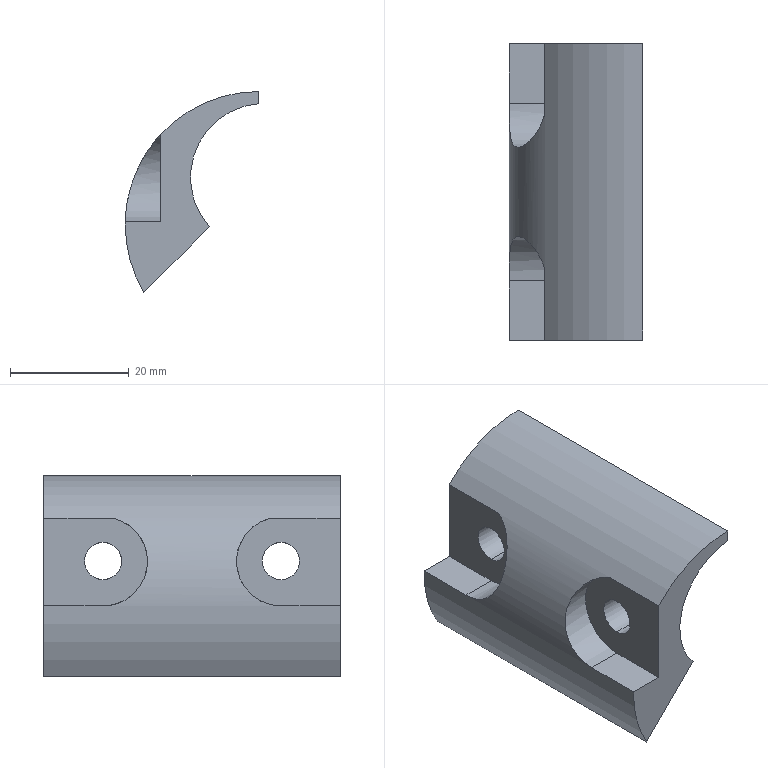Part | SolidWorks | features BaseBody 1 | 1 solid | 16 faces | box 22.5 x 50 x 33.899 mm | volume 12325 mm3 | cylinder 8 | plane 8 | commonest cylinder face diameters 6.3 x4 15 x2 25 x1 45 x1
STEP:
#1=CARTESIAN_POINT('',(909.83,-3885.973,891.894));
#2=VERTEX_POINT('',#1);
#3=CARTESIAN_POINT('',(909.868,-3885.973,898.194));
#4=VERTEX_POINT('',#3);
#5=CARTESIAN_POINT('',(909.83,-3885.973,891.894));
#6=CARTESIAN_POINT('',(909.83,-3886.182,891.894));
#7=CARTESIAN_POINT('',(909.825,-3886.387,891.915));
#8=CARTESIAN_POINT('',(909.805,-3886.791,891.995));
#9=CARTESIAN_POINT('',(909.79,-3886.992,892.056));
#10=CARTESIAN_POINT('',(909.753,-3887.373,892.214));
#11=CARTESIAN_POINT('',(909.731,-3887.553,892.311));
#12=CARTESIAN_POINT('',(909.684,-3887.895,892.54));
#13=CARTESIAN_POINT('',(909.658,-3888.056,892.672));
#14=CARTESIAN_POINT('',(909.607,-3888.346,892.962));
#15=CARTESIAN_POINT('',(909.582,-3888.476,893.12));
#16=CARTESIAN_POINT('',(909.536,-3888.706,893.464));
#17=CARTESIAN_POINT('',(909.515,-3888.804,893.646));
#18=CARTESIAN_POINT('',(909.48,-3888.961,894.025));
#19=CARTESIAN_POINT('',(909.466,-3889.022,894.225));
#20=CARTESIAN_POINT('',(909.448,-3889.103,894.632));
#21=CARTESIAN_POINT('',(909.444,-3889.123,894.839));
#22=CARTESIAN_POINT('',(909.447,-3889.123,895.257));
#23=CARTESIAN_POINT('',(909.454,-3889.102,895.462));
#24=CARTESIAN_POINT('',(909.476,-3889.021,895.866));
#25=CARTESIAN_POINT('',(909.492,-3888.96,896.066));
#26=CARTESIAN_POINT('',(909.531,-3888.801,896.447));
#27=CARTESIAN_POINT('',(909.554,-3888.704,896.627));
#28=CARTESIAN_POINT('',(909.605,-3888.475,896.968));
#29=CARTESIAN_POINT('',(909.632,-3888.343,897.129));
#30=CARTESIAN_POINT('',(909.686,-3888.053,897.418));
#31=CARTESIAN_POINT('',(909.713,-3887.895,897.548));
#32=CARTESIAN_POINT('',(909.764,-3887.551,897.778));
#33=CARTESIAN_POINT('',(909.787,-3887.369,897.875));
#34=CARTESIAN_POINT('',(909.826,-3886.991,898.032));
#35=CARTESIAN_POINT('',(909.841,-3886.791,898.093));
#36=CARTESIAN_POINT('',(909.863,-3886.384,898.174));
#37=CARTESIAN_POINT('',(909.868,-3886.179,898.194));
#38=CARTESIAN_POINT('',(909.868,-3885.973,898.194));
#39=B_SPLINE_CURVE_WITH_KNOTS('',3,(#5,#6,#7,#8,#9,#10,#11,#12,#13,#14,#15,#16,#17,#18,#19,#20,#21,#22,#23,#24,#25,#26,#27,#28,#29,#30,#31,#32,#33,#34,#35,#36,#37,#38),.UNSPECIFIED.,.F.,.F.,(4,2,2,2,2,2,2,2,2,2,2,2,2,2,2,2,4),(0.,0.0006179,0.001236,0.001854,0.002472,0.00309,0.003707,0.004325,0.004943,0.005561,0.006179,0.006797,0.007415,0.008033,0.008651,0.009269,0.009886),.UNSPECIFIED.);
#40=EDGE_CURVE('',#2,#4,#39,.T.);
#41=ORIENTED_EDGE('',*,*,#40,.F.);
#42=CARTESIAN_POINT('',(904.446,-3885.973,891.894));
#43=VERTEX_POINT('',#42);
#44=CARTESIAN_POINT('',(894.755,-3885.973,891.894));
#45=DIRECTION('',(-1.,0.,0.));
#46=VECTOR('',#45,1000.);
#47=LINE('',#44,#46);
#48=EDGE_CURVE('',#2,#43,#47,.T.);
#49=ORIENTED_EDGE('',*,*,#48,.T.);
#50=CARTESIAN_POINT('',(904.446,-3885.973,898.194));
#51=VERTEX_POINT('',#50);
#52=CARTESIAN_POINT('',(904.446,-3885.973,895.044));
#53=DIRECTION('',(-1.,0.,0.));
#54=DIRECTION('',(0.,0.,1.));
#55=AXIS2_PLACEMENT_3D('',#52,#53,#54);
#56=CIRCLE('',#55,3.15);
#57=EDGE_CURVE('',#43,#51,#56,.T.);
#58=ORIENTED_EDGE('',*,*,#57,.T.);
#59=CARTESIAN_POINT('',(894.755,-3885.973,898.194));
#60=DIRECTION('',(-1.,0.,0.));
#61=VECTOR('',#60,1000.);
#62=LINE('',#59,#61);
#63=EDGE_CURVE('',#4,#51,#62,.T.);
#64=ORIENTED_EDGE('',*,*,#63,.F.);
#65=EDGE_LOOP('',(#41,#49,#58,#64));
#66=FACE_OUTER_BOUND('',#65,.T.);
#67=CARTESIAN_POINT('',(894.755,-3885.973,895.044));
#68=DIRECTION('',(-1.,0.,0.));
#69=DIRECTION('',(0.,0.,1.));
#70=AXIS2_PLACEMENT_3D('',#67,#68,#69);
#71=CYLINDRICAL_SURFACE('',#70,3.15);
#72=ADVANCED_FACE('',(#66),#71,.F.);
#73=CARTESIAN_POINT('',(904.446,-3915.973,891.894));
#74=VERTEX_POINT('',#73);
#75=CARTESIAN_POINT('',(904.446,-3915.973,898.194));
#76=VERTEX_POINT('',#75);
#77=CARTESIAN_POINT('',(904.446,-3915.973,895.044));
#78=DIRECTION('',(-1.,0.,0.));
#79=DIRECTION('',(0.,0.,-1.));
#80=AXIS2_PLACEMENT_3D('',#77,#78,#79);
#81=CIRCLE('',#80,3.15);
#82=EDGE_CURVE('',#74,#76,#81,.T.);
#83=ORIENTED_EDGE('',*,*,#82,.T.);
#84=CARTESIAN_POINT('',(909.868,-3915.973,898.194));
#85=VERTEX_POINT('',#84);
#86=CARTESIAN_POINT('',(894.755,-3915.973,898.194));
#87=DIRECTION('',(1.,0.,0.));
#88=VECTOR('',#87,1000.);
#89=LINE('',#86,#88);
#90=EDGE_CURVE('',#76,#85,#89,.T.);
#91=ORIENTED_EDGE('',*,*,#90,.T.);
#92=CARTESIAN_POINT('',(909.83,-3915.973,891.894));
#93=VERTEX_POINT('',#92);
#94=CARTESIAN_POINT('',(909.83,-3915.973,891.894));
#95=CARTESIAN_POINT('',(909.83,-3916.179,891.894));
#96=CARTESIAN_POINT('',(909.825,-3916.389,891.915));
#97=CARTESIAN_POINT('',(909.805,-3916.793,891.996));
#98=CARTESIAN_POINT('',(909.79,-3916.99,892.055));
#99=CARTESIAN_POINT('',(909.735,-3917.563,892.293));
#100=CARTESIAN_POINT('',(909.684,-3917.909,892.525));
#101=CARTESIAN_POINT('',(909.607,-3918.347,892.963));
#102=CARTESIAN_POINT('',(909.582,-3918.476,893.121));
#103=CARTESIAN_POINT('',(909.536,-3918.704,893.461));
#104=CARTESIAN_POINT('',(909.515,-3918.803,893.646));
#105=CARTESIAN_POINT('',(909.48,-3918.961,894.026));
#106=CARTESIAN_POINT('',(909.466,-3919.021,894.222));
#107=CARTESIAN_POINT('',(909.449,-3919.102,894.628));
#108=CARTESIAN_POINT('',(909.445,-3919.123,894.837));
#109=CARTESIAN_POINT('',(909.447,-3919.123,895.255));
#110=CARTESIAN_POINT('',(909.453,-3919.102,895.46));
#111=CARTESIAN_POINT('',(909.476,-3919.022,895.863));
#112=CARTESIAN_POINT('',(909.492,-3918.961,896.064));
#113=CARTESIAN_POINT('',(909.531,-3918.802,896.444));
#114=CARTESIAN_POINT('',(909.554,-3918.706,896.625));
#115=CARTESIAN_POINT('',(909.604,-3918.477,896.966));
#116=CARTESIAN_POINT('',(909.632,-3918.345,897.127));
#117=CARTESIAN_POINT('',(909.686,-3918.056,897.416));
#118=CARTESIAN_POINT('',(909.713,-3917.898,897.546));
#119=CARTESIAN_POINT('',(909.764,-3917.555,897.776));
#120=CARTESIAN_POINT('',(909.787,-3917.373,897.873));
#121=CARTESIAN_POINT('',(909.825,-3916.995,898.031));
#122=CARTESIAN_POINT('',(909.841,-3916.796,898.092));
#123=CARTESIAN_POINT('',(909.863,-3916.388,898.173));
#124=CARTESIAN_POINT('',(909.868,-3916.182,898.194));
#125=CARTESIAN_POINT('',(909.868,-3915.973,898.194));
#126=B_SPLINE_CURVE_WITH_KNOTS('',3,(#94,#95,#96,#97,#98,#99,#100,#101,#102,#103,#104,#105,#106,#107,#108,#109,#110,#111,#112,#113,#114,#115,#116,#117,#118,#119,#120,#121,#122,#123,#124,#125),.UNSPECIFIED.,.F.,.F.,(4,2,2,2,2,2,2,2,2,2,2,2,2,2,2,4),(-0.004938,-0.004321,-0.003703,-0.002468,-0.001851,-0.001233,-0.0006155,0.000002039,0.0006196,0.001237,0.001855,0.002472,0.00309,0.003707,0.004325,0.004942),.UNSPECIFIED.);
#127=EDGE_CURVE('',#93,#85,#126,.T.);
#128=ORIENTED_EDGE('',*,*,#127,.F.);
#129=CARTESIAN_POINT('',(894.755,-3915.973,891.894));
#130=DIRECTION('',(1.,0.,0.));
#131=VECTOR('',#130,1000.);
#132=LINE('',#129,#131);
#133=EDGE_CURVE('',#74,#93,#132,.T.);
#134=ORIENTED_EDGE('',*,*,#133,.F.);
#135=EDGE_LOOP('',(#83,#91,#128,#134));
#136=FACE_OUTER_BOUND('',#135,.T.);
#137=CARTESIAN_POINT('',(894.755,-3915.973,895.044));
#138=DIRECTION('',(1.,0.,0.));
#139=DIRECTION('',(0.,0.,-1.));
#140=AXIS2_PLACEMENT_3D('',#137,#138,#139);
#141=CYLINDRICAL_SURFACE('',#140,3.15);
#142=ADVANCED_FACE('',(#136),#141,.F.);
#143=CARTESIAN_POINT('',(904.446,-3875.973,902.268));
#144=VERTEX_POINT('',#143);
#145=CARTESIAN_POINT('',(904.446,-3887.706,902.268));
#146=VERTEX_POINT('',#145);
#147=CARTESIAN_POINT('',(904.446,-3875.973,902.268));
#148=DIRECTION('',(0.,-1.,0.));
#149=VECTOR('',#148,1000.);
#150=LINE('',#147,#149);
#151=EDGE_CURVE('',#144,#146,#150,.T.);
#152=ORIENTED_EDGE('',*,*,#151,.T.);
#153=CARTESIAN_POINT('',(898.451,-3885.973,887.471));
#154=VERTEX_POINT('',#153);
#155=CARTESIAN_POINT('',(904.446,-3887.706,902.268));
#156=CARTESIAN_POINT('',(904.344,-3888.167,902.159));
#157=CARTESIAN_POINT('',(904.209,-3888.6,902.011));
#158=CARTESIAN_POINT('',(903.969,-3889.215,901.738));
#159=CARTESIAN_POINT('',(903.883,-3889.414,901.639));
#160=CARTESIAN_POINT('',(903.701,-3889.802,901.424));
#161=CARTESIAN_POINT('',(903.604,-3889.991,901.308));
#162=CARTESIAN_POINT('',(903.305,-3890.534,900.941));
#163=CARTESIAN_POINT('',(903.093,-3890.867,900.671));
#164=CARTESIAN_POINT('',(902.655,-3891.481,900.08));
#165=CARTESIAN_POINT('',(902.427,-3891.763,899.758));
#166=CARTESIAN_POINT('',(901.976,-3892.263,899.079));
#167=CARTESIAN_POINT('',(901.752,-3892.483,898.721));
#168=CARTESIAN_POINT('',(901.309,-3892.863,897.965));
#169=CARTESIAN_POINT('',(901.089,-3893.024,897.563));
#170=CARTESIAN_POINT('',(900.672,-3893.274,896.74));
#171=CARTESIAN_POINT('',(900.473,-3893.364,896.318));
#172=CARTESIAN_POINT('',(900.193,-3893.444,895.668));
#173=CARTESIAN_POINT('',(900.102,-3893.461,895.449));
#174=CARTESIAN_POINT('',(899.927,-3893.476,895.004));
#175=CARTESIAN_POINT('',(899.842,-3893.474,894.777));
#176=CARTESIAN_POINT('',(899.599,-3893.436,894.099));
#177=CARTESIAN_POINT('',(899.455,-3893.37,893.65));
#178=CARTESIAN_POINT('',(899.262,-3893.208,892.983));
#179=CARTESIAN_POINT('',(899.202,-3893.144,892.762));
#180=CARTESIAN_POINT('',(899.09,-3892.994,892.322));
#181=CARTESIAN_POINT('',(899.037,-3892.907,892.102));
#182=CARTESIAN_POINT('',(898.893,-3892.615,891.457));
#183=CARTESIAN_POINT('',(898.814,-3892.382,891.048));
#184=CARTESIAN_POINT('',(898.718,-3891.975,890.467));
#185=CARTESIAN_POINT('',(898.689,-3891.829,890.28));
#186=CARTESIAN_POINT('',(898.638,-3891.518,889.916));
#187=CARTESIAN_POINT('',(898.616,-3891.352,889.74));
#188=CARTESIAN_POINT('',(898.558,-3890.836,889.242));
#189=CARTESIAN_POINT('',(898.531,-3890.464,888.945));
#190=CARTESIAN_POINT('',(898.501,-3889.861,888.554));
#191=CARTESIAN_POINT('',(898.493,-3889.652,888.431));
#192=CARTESIAN_POINT('',(898.479,-3889.225,888.209));
#193=CARTESIAN_POINT('',(898.474,-3889.007,888.109));
#194=CARTESIAN_POINT('',(898.462,-3888.343,887.84));
#195=CARTESIAN_POINT('',(898.457,-3887.886,887.703));
#196=CARTESIAN_POINT('',(898.452,-3886.939,887.518));
#197=CARTESIAN_POINT('',(898.451,-3886.457,887.471));
#198=CARTESIAN_POINT('',(898.451,-3885.973,887.471));
#199=B_SPLINE_CURVE_WITH_KNOTS('',3,(#155,#156,#157,#158,#159,#160,#161,#162,#163,#164,#165,#166,#167,#168,#169,#170,#171,#172,#173,#174,#175,#176,#177,#178,#179,#180,#181,#182,#183,#184,#185,#186,#187,#188,#189,#190,#191,#192,#193,#194,#195,#196,#197,#198),.UNSPECIFIED.,.F.,.F.,(4,2,2,2,2,2,2,2,2,2,2,2,2,2,2,2,2,2,2,2,2,4),(0.,0.001427,0.002141,0.002855,0.004282,0.005709,0.007137,0.008564,0.009991,0.01071,0.01142,0.01285,0.01356,0.01427,0.0157,0.01641,0.01713,0.01856,0.01927,0.01998,0.02141,0.02284),.UNSPECIFIED.);
#200=EDGE_CURVE('',#146,#154,#199,.T.);
#201=ORIENTED_EDGE('',*,*,#200,.T.);
#202=CARTESIAN_POINT('',(898.451,-3875.973,887.471));
#203=VERTEX_POINT('',#202);
#204=CARTESIAN_POINT('',(898.451,-3875.973,887.471));
#205=DIRECTION('',(0.,1.,0.));
#206=VECTOR('',#205,1000.);
#207=LINE('',#204,#206);
#208=EDGE_CURVE('',#154,#203,#207,.T.);
#209=ORIENTED_EDGE('',*,*,#208,.T.);
#210=CARTESIAN_POINT('',(901.547,-3875.973,875.573));
#211=VERTEX_POINT('',#210);
#212=CARTESIAN_POINT('',(920.946,-3875.973,886.971));
#213=DIRECTION('',(0.,-1.,0.));
#214=DIRECTION('',(0.,0.,-1.));
#215=AXIS2_PLACEMENT_3D('',#212,#213,#214);
#216=CIRCLE('',#215,22.5);
#217=EDGE_CURVE('',#203,#211,#216,.T.);
#218=ORIENTED_EDGE('',*,*,#217,.T.);
#219=CARTESIAN_POINT('',(901.547,-3925.973,875.573));
#220=VERTEX_POINT('',#219);
#221=CARTESIAN_POINT('',(901.547,-3875.973,875.573));
#222=DIRECTION('',(0.,-1.,0.));
#223=VECTOR('',#222,1000.);
#224=LINE('',#221,#223);
#225=EDGE_CURVE('',#211,#220,#224,.T.);
#226=ORIENTED_EDGE('',*,*,#225,.T.);
#227=CARTESIAN_POINT('',(898.451,-3925.973,887.471));
#228=VERTEX_POINT('',#227);
#229=CARTESIAN_POINT('',(920.946,-3925.973,886.971));
#230=DIRECTION('',(0.,1.,0.));
#231=DIRECTION('',(0.,0.,-1.));
#232=AXIS2_PLACEMENT_3D('',#229,#230,#231);
#233=CIRCLE('',#232,22.5);
#234=EDGE_CURVE('',#220,#228,#233,.T.);
#235=ORIENTED_EDGE('',*,*,#234,.T.);
#236=CARTESIAN_POINT('',(898.451,-3915.973,887.471));
#237=VERTEX_POINT('',#236);
#238=CARTESIAN_POINT('',(898.451,-3875.973,887.471));
#239=DIRECTION('',(0.,1.,0.));
#240=VECTOR('',#239,1000.);
#241=LINE('',#238,#240);
#242=EDGE_CURVE('',#228,#237,#241,.T.);
#243=ORIENTED_EDGE('',*,*,#242,.T.);
#244=CARTESIAN_POINT('',(904.446,-3914.24,902.268));
#245=VERTEX_POINT('',#244);
#246=CARTESIAN_POINT('',(898.451,-3915.973,887.471));
#247=CARTESIAN_POINT('',(898.451,-3915.49,887.471));
#248=CARTESIAN_POINT('',(898.452,-3915.014,887.518));
#249=CARTESIAN_POINT('',(898.456,-3914.313,887.654));
#250=CARTESIAN_POINT('',(898.458,-3914.081,887.71));
#251=CARTESIAN_POINT('',(898.462,-3913.62,887.846));
#252=CARTESIAN_POINT('',(898.466,-3913.391,887.926));
#253=CARTESIAN_POINT('',(898.478,-3912.724,888.195));
#254=CARTESIAN_POINT('',(898.49,-3912.301,888.415));
#255=CARTESIAN_POINT('',(898.53,-3911.499,888.933));
#256=CARTESIAN_POINT('',(898.557,-3911.118,889.235));
#257=CARTESIAN_POINT('',(898.634,-3910.432,889.895));
#258=CARTESIAN_POINT('',(898.683,-3910.123,890.255));
#259=CARTESIAN_POINT('',(898.779,-3909.711,890.837));
#260=CARTESIAN_POINT('',(898.815,-3909.582,891.039));
#261=CARTESIAN_POINT('',(898.895,-3909.347,891.45));
#262=CARTESIAN_POINT('',(898.938,-3909.24,891.659));
#263=CARTESIAN_POINT('',(899.081,-3908.95,892.298));
#264=CARTESIAN_POINT('',(899.192,-3908.799,892.737));
#265=CARTESIAN_POINT('',(899.452,-3908.577,893.641));
#266=CARTESIAN_POINT('',(899.597,-3908.511,894.092));
#267=CARTESIAN_POINT('',(899.837,-3908.473,894.765));
#268=CARTESIAN_POINT('',(899.921,-3908.47,894.989));
#269=CARTESIAN_POINT('',(900.097,-3908.484,895.436));
#270=CARTESIAN_POINT('',(900.189,-3908.501,895.659));
#271=CARTESIAN_POINT('',(900.472,-3908.581,896.316));
#272=CARTESIAN_POINT('',(900.672,-3908.672,896.74));
#273=CARTESIAN_POINT('',(901.089,-3908.922,897.564));
#274=CARTESIAN_POINT('',(901.309,-3909.083,897.965));
#275=CARTESIAN_POINT('',(901.753,-3909.465,898.722));
#276=CARTESIAN_POINT('',(901.977,-3909.685,899.08));
#277=CARTESIAN_POINT('',(902.428,-3910.185,899.759));
#278=CARTESIAN_POINT('',(902.656,-3910.467,900.081));
#279=CARTESIAN_POINT('',(903.093,-3911.079,900.67));
#280=CARTESIAN_POINT('',(903.303,-3911.41,900.939));
#281=CARTESIAN_POINT('',(903.599,-3911.946,901.302));
#282=CARTESIAN_POINT('',(903.695,-3912.132,901.417));
#283=CARTESIAN_POINT('',(903.877,-3912.519,901.632));
#284=CARTESIAN_POINT('',(903.965,-3912.721,901.734));
#285=CARTESIAN_POINT('',(904.208,-3913.344,902.01));
#286=CARTESIAN_POINT('',(904.344,-3913.779,902.159));
#287=CARTESIAN_POINT('',(904.446,-3914.24,902.268));
#288=B_SPLINE_CURVE_WITH_KNOTS('',3,(#246,#247,#248,#249,#250,#251,#252,#253,#254,#255,#256,#257,#258,#259,#260,#261,#262,#263,#264,#265,#266,#267,#268,#269,#270,#271,#272,#273,#274,#275,#276,#277,#278,#279,#280,#281,#282,#283,#284,#285,#286,#287),.UNSPECIFIED.,.F.,.F.,(4,2,2,2,2,2,2,2,2,2,2,2,2,2,2,2,2,2,2,2,4),(0.,0.001429,0.002144,0.002859,0.004288,0.005718,0.007147,0.007862,0.008576,0.01001,0.01144,0.01215,0.01286,0.01429,0.01572,0.01715,0.01858,0.02001,0.02073,0.02144,0.02287),.UNSPECIFIED.);
#289=EDGE_CURVE('',#237,#245,#288,.T.);
#290=ORIENTED_EDGE('',*,*,#289,.T.);
#291=CARTESIAN_POINT('',(904.446,-3925.973,902.268));
#292=VERTEX_POINT('',#291);
#293=CARTESIAN_POINT('',(904.446,-3875.973,902.268));
#294=DIRECTION('',(0.,-1.,0.));
#295=VECTOR('',#294,1000.);
#296=LINE('',#293,#295);
#297=EDGE_CURVE('',#245,#292,#296,.T.);
#298=ORIENTED_EDGE('',*,*,#297,.T.);
#299=CARTESIAN_POINT('',(920.946,-3925.973,909.471));
#300=VERTEX_POINT('',#299);
#301=CARTESIAN_POINT('',(920.946,-3925.973,886.971));
#302=DIRECTION('',(0.,1.,0.));
#303=DIRECTION('',(0.,0.,-1.));
#304=AXIS2_PLACEMENT_3D('',#301,#302,#303);
#305=CIRCLE('',#304,22.5);
#306=EDGE_CURVE('',#292,#300,#305,.T.);
#307=ORIENTED_EDGE('',*,*,#306,.T.);
#308=CARTESIAN_POINT('',(920.946,-3875.973,909.471));
#309=VERTEX_POINT('',#308);
#310=CARTESIAN_POINT('',(920.946,-3875.973,909.471));
#311=DIRECTION('',(0.,1.,0.));
#312=VECTOR('',#311,1000.);
#313=LINE('',#310,#312);
#314=EDGE_CURVE('',#300,#309,#313,.T.);
#315=ORIENTED_EDGE('',*,*,#314,.T.);
#316=CARTESIAN_POINT('',(920.946,-3875.973,886.971));
#317=DIRECTION('',(0.,-1.,0.));
#318=DIRECTION('',(0.,0.,-1.));
#319=AXIS2_PLACEMENT_3D('',#316,#317,#318);
#320=CIRCLE('',#319,22.5);
#321=EDGE_CURVE('',#309,#144,#320,.T.);
#322=ORIENTED_EDGE('',*,*,#321,.T.);
#323=EDGE_LOOP('',(#152,#201,#209,#218,#226,#235,#243,#290,#298,#307,#315,#322));
#324=FACE_OUTER_BOUND('',#323,.T.);
#325=CARTESIAN_POINT('',(920.946,-3875.973,886.971));
#326=DIRECTION('',(0.,-1.,0.));
#327=DIRECTION('',(0.,0.,-1.));
#328=AXIS2_PLACEMENT_3D('',#325,#326,#327);
#329=CYLINDRICAL_SURFACE('',#328,22.5);
#330=ADVANCED_FACE('',(#324),#329,.T.);
#331=CARTESIAN_POINT('',(904.446,-3885.973,887.471));
#332=VERTEX_POINT('',#331);
#333=CARTESIAN_POINT('',(904.446,-3885.973,894.971));
#334=DIRECTION('',(-1.,0.,0.));
#335=DIRECTION('',(0.,0.,1.));
#336=AXIS2_PLACEMENT_3D('',#333,#334,#335);
#337=CIRCLE('',#336,7.5);
#338=EDGE_CURVE('',#332,#146,#337,.T.);
#339=ORIENTED_EDGE('',*,*,#338,.F.);
#340=CARTESIAN_POINT('',(904.446,-3885.973,887.471));
#341=DIRECTION('',(1.,0.,0.));
#342=VECTOR('',#341,1000.);
#343=LINE('',#340,#342);
#344=EDGE_CURVE('',#154,#332,#343,.T.);
#345=ORIENTED_EDGE('',*,*,#344,.F.);
#346=ORIENTED_EDGE('',*,*,#200,.F.);
#347=EDGE_LOOP('',(#339,#345,#346));
#348=FACE_OUTER_BOUND('',#347,.T.);
#349=CARTESIAN_POINT('',(904.446,-3885.973,894.971));
#350=DIRECTION('',(-1.,0.,0.));
#351=DIRECTION('',(0.,0.,1.));
#352=AXIS2_PLACEMENT_3D('',#349,#350,#351);
#353=CYLINDRICAL_SURFACE('',#352,7.5);
#354=ADVANCED_FACE('',(#348),#353,.F.);
#355=CARTESIAN_POINT('',(904.446,-3885.973,895.044));
#356=DIRECTION('',(-1.,0.,0.));
#357=DIRECTION('',(0.,0.,1.));
#358=AXIS2_PLACEMENT_3D('',#355,#356,#357);
#359=CIRCLE('',#358,3.15);
#360=EDGE_CURVE('',#51,#43,#359,.T.);
#361=ORIENTED_EDGE('',*,*,#360,.F.);
#362=ORIENTED_EDGE('',*,*,#57,.F.);
#363=EDGE_LOOP('',(#361,#362));
#364=FACE_BOUND('',#363,.T.);
#365=CARTESIAN_POINT('',(904.446,-3875.973,887.471));
#366=VERTEX_POINT('',#365);
#367=CARTESIAN_POINT('',(904.446,-3876.427,887.471));
#368=DIRECTION('',(0.,1.,0.));
#369=VECTOR('',#368,1000.);
#370=LINE('',#367,#369);
#371=EDGE_CURVE('',#332,#366,#370,.T.);
#372=ORIENTED_EDGE('',*,*,#371,.F.);
#373=ORIENTED_EDGE('',*,*,#338,.T.);
#374=ORIENTED_EDGE('',*,*,#151,.F.);
#375=CARTESIAN_POINT('',(904.446,-3875.973,894.971));
#376=DIRECTION('',(0.,0.,1.));
#377=VECTOR('',#376,1000.);
#378=LINE('',#375,#377);
#379=EDGE_CURVE('',#366,#144,#378,.T.);
#380=ORIENTED_EDGE('',*,*,#379,.F.);
#381=EDGE_LOOP('',(#372,#373,#374,#380));
#382=FACE_OUTER_BOUND('',#381,.T.);
#383=CARTESIAN_POINT('',(904.446,-3876.427,894.971));
#384=DIRECTION('',(1.,0.,0.));
#385=DIRECTION('',(0.,0.,-1.));
#386=AXIS2_PLACEMENT_3D('',#383,#384,#385);
#387=PLANE('',#386);
#388=ADVANCED_FACE('',(#364,#382),#387,.F.);
#389=CARTESIAN_POINT('',(912.621,-3875.973,886.647));
#390=VERTEX_POINT('',#389);
#391=CARTESIAN_POINT('',(912.621,-3875.973,886.647));
#392=DIRECTION('',(-0.7071,0.,-0.7071));
#393=VECTOR('',#392,1000.);
#394=LINE('',#391,#393);
#395=EDGE_CURVE('',#390,#211,#394,.T.);
#396=ORIENTED_EDGE('',*,*,#395,.T.);
#397=ORIENTED_EDGE('',*,*,#217,.F.);
#398=CARTESIAN_POINT('',(908.173,-3875.973,887.471));
#399=DIRECTION('',(1.,0.,0.));
#400=VECTOR('',#399,1000.);
#401=LINE('',#398,#400);
#402=EDGE_CURVE('',#203,#366,#401,.T.);
#403=ORIENTED_EDGE('',*,*,#402,.T.);
#404=ORIENTED_EDGE('',*,*,#379,.T.);
#405=ORIENTED_EDGE('',*,*,#321,.F.);
#406=CARTESIAN_POINT('',(920.946,-3875.973,907.431));
#407=VERTEX_POINT('',#406);
#408=CARTESIAN_POINT('',(920.946,-3875.973,894.564));
#409=DIRECTION('',(0.,0.,-1.));
#410=VECTOR('',#409,1000.);
#411=LINE('',#408,#410);
#412=EDGE_CURVE('',#309,#407,#411,.T.);
#413=ORIENTED_EDGE('',*,*,#412,.T.);
#414=CARTESIAN_POINT('',(921.946,-3875.973,894.971));
#415=DIRECTION('',(0.,-1.,0.));
#416=DIRECTION('',(0.,0.,-1.));
#417=AXIS2_PLACEMENT_3D('',#414,#415,#416);
#418=CIRCLE('',#417,12.5);
#419=EDGE_CURVE('',#407,#390,#418,.T.);
#420=ORIENTED_EDGE('',*,*,#419,.T.);
#421=EDGE_LOOP('',(#396,#397,#403,#404,#405,#413,#420));
#422=FACE_OUTER_BOUND('',#421,.T.);
#423=CARTESIAN_POINT('',(908.173,-3875.973,894.564));
#424=DIRECTION('',(0.,1.,0.));
#425=DIRECTION('',(0.,0.,1.));
#426=AXIS2_PLACEMENT_3D('',#423,#424,#425);
#427=PLANE('',#426);
#428=ADVANCED_FACE('',(#422),#427,.T.);
#429=ORIENTED_EDGE('',*,*,#412,.F.);
#430=ORIENTED_EDGE('',*,*,#314,.F.);
#431=CARTESIAN_POINT('',(920.946,-3925.973,907.431));
#432=VERTEX_POINT('',#431);
#433=CARTESIAN_POINT('',(920.946,-3925.973,909.471));
#434=DIRECTION('',(0.,0.,-1.));
#435=VECTOR('',#434,1000.);
#436=LINE('',#433,#435);
#437=EDGE_CURVE('',#300,#432,#436,.T.);
#438=ORIENTED_EDGE('',*,*,#437,.T.);
#439=CARTESIAN_POINT('',(920.946,-3875.973,907.431));
#440=DIRECTION('',(0.,1.,0.));
#441=VECTOR('',#440,1000.);
#442=LINE('',#439,#441);
#443=EDGE_CURVE('',#432,#407,#442,.T.);
#444=ORIENTED_EDGE('',*,*,#443,.T.);
#445=EDGE_LOOP('',(#429,#430,#438,#444));
#446=FACE_OUTER_BOUND('',#445,.T.);
#447=CARTESIAN_POINT('',(920.946,-3875.973,909.471));
#448=DIRECTION('',(1.,0.,0.));
#449=DIRECTION('',(0.,0.,-1.));
#450=AXIS2_PLACEMENT_3D('',#447,#448,#449);
#451=PLANE('',#450);
#452=ADVANCED_FACE('',(#446),#451,.T.);
#453=CARTESIAN_POINT('',(904.446,-3925.973,887.471));
#454=VERTEX_POINT('',#453);
#455=CARTESIAN_POINT('',(908.173,-3925.973,887.471));
#456=DIRECTION('',(1.,0.,0.));
#457=VECTOR('',#456,1000.);
#458=LINE('',#455,#457);
#459=EDGE_CURVE('',#228,#454,#458,.T.);
#460=ORIENTED_EDGE('',*,*,#459,.F.);
#461=ORIENTED_EDGE('',*,*,#234,.F.);
#462=CARTESIAN_POINT('',(912.621,-3925.973,886.647));
#463=VERTEX_POINT('',#462);
#464=CARTESIAN_POINT('',(912.621,-3925.973,886.647));
#465=DIRECTION('',(-0.7071,0.,-0.7071));
#466=VECTOR('',#465,1000.);
#467=LINE('',#464,#466);
#468=EDGE_CURVE('',#463,#220,#467,.T.);
#469=ORIENTED_EDGE('',*,*,#468,.F.);
#470=CARTESIAN_POINT('',(921.946,-3925.973,894.971));
#471=DIRECTION('',(0.,-1.,0.));
#472=DIRECTION('',(0.,0.,-1.));
#473=AXIS2_PLACEMENT_3D('',#470,#471,#472);
#474=CIRCLE('',#473,12.5);
#475=EDGE_CURVE('',#432,#463,#474,.T.);
#476=ORIENTED_EDGE('',*,*,#475,.F.);
#477=ORIENTED_EDGE('',*,*,#437,.F.);
#478=ORIENTED_EDGE('',*,*,#306,.F.);
#479=CARTESIAN_POINT('',(904.446,-3925.973,894.564));
#480=DIRECTION('',(0.,0.,1.));
#481=VECTOR('',#480,1000.);
#482=LINE('',#479,#481);
#483=EDGE_CURVE('',#454,#292,#482,.T.);
#484=ORIENTED_EDGE('',*,*,#483,.F.);
#485=EDGE_LOOP('',(#460,#461,#469,#476,#477,#478,#484));
#486=FACE_OUTER_BOUND('',#485,.T.);
#487=CARTESIAN_POINT('',(908.173,-3925.973,894.564));
#488=DIRECTION('',(0.,1.,0.));
#489=DIRECTION('',(0.,0.,1.));
#490=AXIS2_PLACEMENT_3D('',#487,#488,#489);
#491=PLANE('',#490);
#492=ADVANCED_FACE('',(#486),#491,.F.);
#493=ORIENTED_EDGE('',*,*,#82,.F.);
#494=CARTESIAN_POINT('',(904.446,-3915.973,895.044));
#495=DIRECTION('',(-1.,0.,0.));
#496=DIRECTION('',(0.,0.,-1.));
#497=AXIS2_PLACEMENT_3D('',#494,#495,#496);
#498=CIRCLE('',#497,3.15);
#499=EDGE_CURVE('',#76,#74,#498,.T.);
#500=ORIENTED_EDGE('',*,*,#499,.F.);
#501=EDGE_LOOP('',(#493,#500));
#502=FACE_BOUND('',#501,.T.);
#503=ORIENTED_EDGE('',*,*,#297,.F.);
#504=CARTESIAN_POINT('',(904.446,-3915.973,887.471));
#505=VERTEX_POINT('',#504);
#506=CARTESIAN_POINT('',(904.446,-3915.973,894.971));
#507=DIRECTION('',(1.,0.,0.));
#508=DIRECTION('',(0.,0.,-1.));
#509=AXIS2_PLACEMENT_3D('',#506,#507,#508);
#510=CIRCLE('',#509,7.5);
#511=EDGE_CURVE('',#505,#245,#510,.T.);
#512=ORIENTED_EDGE('',*,*,#511,.F.);
#513=CARTESIAN_POINT('',(904.446,-3925.52,887.471));
#514=DIRECTION('',(0.,1.,0.));
#515=VECTOR('',#514,1000.);
#516=LINE('',#513,#515);
#517=EDGE_CURVE('',#454,#505,#516,.T.);
#518=ORIENTED_EDGE('',*,*,#517,.F.);
#519=ORIENTED_EDGE('',*,*,#483,.T.);
#520=EDGE_LOOP('',(#503,#512,#518,#519));
#521=FACE_OUTER_BOUND('',#520,.T.);
#522=CARTESIAN_POINT('',(904.446,-3925.52,894.971));
#523=DIRECTION('',(1.,0.,0.));
#524=DIRECTION('',(0.,0.,-1.));
#525=AXIS2_PLACEMENT_3D('',#522,#523,#524);
#526=PLANE('',#525);
#527=ADVANCED_FACE('',(#502,#521),#526,.F.);
#528=CARTESIAN_POINT('',(904.446,-3915.973,887.471));
#529=DIRECTION('',(-1.,0.,0.));
#530=VECTOR('',#529,1000.);
#531=LINE('',#528,#530);
#532=EDGE_CURVE('',#505,#237,#531,.T.);
#533=ORIENTED_EDGE('',*,*,#532,.F.);
#534=ORIENTED_EDGE('',*,*,#511,.T.);
#535=ORIENTED_EDGE('',*,*,#289,.F.);
#536=EDGE_LOOP('',(#533,#534,#535));
#537=FACE_OUTER_BOUND('',#536,.T.);
#538=CARTESIAN_POINT('',(904.446,-3915.973,894.971));
#539=DIRECTION('',(1.,0.,0.));
#540=DIRECTION('',(0.,0.,-1.));
#541=AXIS2_PLACEMENT_3D('',#538,#539,#540);
#542=CYLINDRICAL_SURFACE('',#541,7.5);
#543=ADVANCED_FACE('',(#537),#542,.F.);
#544=ORIENTED_EDGE('',*,*,#517,.T.);
#545=ORIENTED_EDGE('',*,*,#532,.T.);
#546=ORIENTED_EDGE('',*,*,#242,.F.);
#547=ORIENTED_EDGE('',*,*,#459,.T.);
#548=EDGE_LOOP('',(#544,#545,#546,#547));
#549=FACE_OUTER_BOUND('',#548,.T.);
#550=CARTESIAN_POINT('',(904.446,-3915.973,887.471));
#551=DIRECTION('',(0.,0.,-1.));
#552=DIRECTION('',(0.,1.,0.));
#553=AXIS2_PLACEMENT_3D('',#550,#551,#552);
#554=PLANE('',#553);
#555=ADVANCED_FACE('',(#549),#554,.F.);
#556=ORIENTED_EDGE('',*,*,#395,.F.);
#557=CARTESIAN_POINT('',(912.621,-3875.973,886.647));
#558=DIRECTION('',(0.,-1.,0.));
#559=VECTOR('',#558,1000.);
#560=LINE('',#557,#559);
#561=EDGE_CURVE('',#390,#463,#560,.T.);
#562=ORIENTED_EDGE('',*,*,#561,.T.);
#563=ORIENTED_EDGE('',*,*,#468,.T.);
#564=ORIENTED_EDGE('',*,*,#225,.F.);
#565=EDGE_LOOP('',(#556,#562,#563,#564));
#566=FACE_OUTER_BOUND('',#565,.T.);
#567=CARTESIAN_POINT('',(912.107,-3875.973,886.133));
#568=DIRECTION('',(0.7071,0.,-0.7071));
#569=DIRECTION('',(-0.7071,0.,-0.7071));
#570=AXIS2_PLACEMENT_3D('',#567,#568,#569);
#571=PLANE('',#570);
#572=ADVANCED_FACE('',(#566),#571,.T.);
#573=ORIENTED_EDGE('',*,*,#208,.F.);
#574=ORIENTED_EDGE('',*,*,#344,.T.);
#575=ORIENTED_EDGE('',*,*,#371,.T.);
#576=ORIENTED_EDGE('',*,*,#402,.F.);
#577=EDGE_LOOP('',(#573,#574,#575,#576));
#578=FACE_OUTER_BOUND('',#577,.T.);
#579=CARTESIAN_POINT('',(904.446,-3885.973,887.471));
#580=DIRECTION('',(0.,0.,-1.));
#581=DIRECTION('',(0.,1.,0.));
#582=AXIS2_PLACEMENT_3D('',#579,#580,#581);
#583=PLANE('',#582);
#584=ADVANCED_FACE('',(#578),#583,.F.);
#585=ORIENTED_EDGE('',*,*,#48,.F.);
#586=CARTESIAN_POINT('',(909.868,-3885.973,898.194));
#587=CARTESIAN_POINT('',(909.868,-3885.767,898.194));
#588=CARTESIAN_POINT('',(909.862,-3885.557,898.173));
#589=CARTESIAN_POINT('',(909.841,-3885.153,898.092));
#590=CARTESIAN_POINT('',(909.826,-3884.956,898.033));
#591=CARTESIAN_POINT('',(909.767,-3884.383,897.795));
#592=CARTESIAN_POINT('',(909.714,-3884.038,897.563));
#593=CARTESIAN_POINT('',(909.632,-3883.6,897.126));
#594=CARTESIAN_POINT('',(909.605,-3883.471,896.968));
#595=CARTESIAN_POINT('',(909.555,-3883.243,896.628));
#596=CARTESIAN_POINT('',(909.531,-3883.144,896.444));
#597=CARTESIAN_POINT('',(909.492,-3882.986,896.064));
#598=CARTESIAN_POINT('',(909.476,-3882.926,895.868));
#599=CARTESIAN_POINT('',(909.454,-3882.844,895.463));
#600=CARTESIAN_POINT('',(909.447,-3882.823,895.254));
#601=CARTESIAN_POINT('',(909.445,-3882.823,894.836));
#602=CARTESIAN_POINT('',(909.449,-3882.844,894.631));
#603=CARTESIAN_POINT('',(909.466,-3882.924,894.227));
#604=CARTESIAN_POINT('',(909.48,-3882.985,894.027));
#605=CARTESIAN_POINT('',(909.515,-3883.143,893.646));
#606=CARTESIAN_POINT('',(909.535,-3883.24,893.465));
#607=CARTESIAN_POINT('',(909.582,-3883.468,893.123));
#608=CARTESIAN_POINT('',(909.607,-3883.6,892.962));
#609=CARTESIAN_POINT('',(909.658,-3883.89,892.673));
#610=CARTESIAN_POINT('',(909.683,-3884.047,892.542));
#611=CARTESIAN_POINT('',(909.731,-3884.391,892.312));
#612=CARTESIAN_POINT('',(909.753,-3884.573,892.215));
#613=CARTESIAN_POINT('',(909.79,-3884.952,892.057));
#614=CARTESIAN_POINT('',(909.805,-3885.15,891.996));
#615=CARTESIAN_POINT('',(909.825,-3885.558,891.915));
#616=CARTESIAN_POINT('',(909.83,-3885.764,891.894));
#617=CARTESIAN_POINT('',(909.83,-3885.973,891.894));
#618=B_SPLINE_CURVE_WITH_KNOTS('',3,(#586,#587,#588,#589,#590,#591,#592,#593,#594,#595,#596,#597,#598,#599,#600,#601,#602,#603,#604,#605,#606,#607,#608,#609,#610,#611,#612,#613,#614,#615,#616,#617),.UNSPECIFIED.,.F.,.F.,(4,2,2,2,2,2,2,2,2,2,2,2,2,2,2,4),(0.009886,0.0105,0.01112,0.01236,0.01297,0.01359,0.01421,0.01483,0.01544,0.01606,0.01668,0.0173,0.01791,0.01853,0.01915,0.01977),.UNSPECIFIED.);
#619=EDGE_CURVE('',#4,#2,#618,.T.);
#620=ORIENTED_EDGE('',*,*,#619,.F.);
#621=ORIENTED_EDGE('',*,*,#63,.T.);
#622=ORIENTED_EDGE('',*,*,#360,.T.);
#623=EDGE_LOOP('',(#585,#620,#621,#622));
#624=FACE_OUTER_BOUND('',#623,.T.);
#625=CARTESIAN_POINT('',(894.755,-3885.973,895.044));
#626=DIRECTION('',(-1.,0.,0.));
#627=DIRECTION('',(0.,0.,1.));
#628=AXIS2_PLACEMENT_3D('',#625,#626,#627);
#629=CYLINDRICAL_SURFACE('',#628,3.15);
#630=ADVANCED_FACE('',(#624),#629,.F.);
#631=ORIENTED_EDGE('',*,*,#419,.F.);
#632=ORIENTED_EDGE('',*,*,#443,.F.);
#633=ORIENTED_EDGE('',*,*,#475,.T.);
#634=ORIENTED_EDGE('',*,*,#561,.F.);
#635=EDGE_LOOP('',(#631,#632,#633,#634));
#636=FACE_OUTER_BOUND('',#635,.T.);
#637=ORIENTED_EDGE('',*,*,#127,.T.);
#638=CARTESIAN_POINT('',(909.868,-3915.973,898.194));
#639=CARTESIAN_POINT('',(909.868,-3915.764,898.194));
#640=CARTESIAN_POINT('',(909.863,-3915.559,898.173));
#641=CARTESIAN_POINT('',(909.841,-3915.155,898.093));
#642=CARTESIAN_POINT('',(909.826,-3914.955,898.032));
#643=CARTESIAN_POINT('',(909.787,-3914.574,897.874));
#644=CARTESIAN_POINT('',(909.764,-3914.393,897.777));
#645=CARTESIAN_POINT('',(909.713,-3914.052,897.548));
#646=CARTESIAN_POINT('',(909.686,-3913.891,897.416));
#647=CARTESIAN_POINT('',(909.632,-3913.601,897.127));
#648=CARTESIAN_POINT('',(909.605,-3913.471,896.969));
#649=CARTESIAN_POINT('',(909.554,-3913.241,896.625));
#650=CARTESIAN_POINT('',(909.531,-3913.144,896.444));
#651=CARTESIAN_POINT('',(909.492,-3912.986,896.065));
#652=CARTESIAN_POINT('',(909.476,-3912.925,895.866));
#653=CARTESIAN_POINT('',(909.453,-3912.844,895.459));
#654=CARTESIAN_POINT('',(909.447,-3912.823,895.252));
#655=CARTESIAN_POINT('',(909.445,-3912.823,894.834));
#656=CARTESIAN_POINT('',(909.449,-3912.844,894.629));
#657=CARTESIAN_POINT('',(909.466,-3912.924,894.225));
#658=CARTESIAN_POINT('',(909.48,-3912.986,894.024));
#659=CARTESIAN_POINT('',(909.515,-3913.144,893.643));
#660=CARTESIAN_POINT('',(909.536,-3913.241,893.463));
#661=CARTESIAN_POINT('',(909.582,-3913.47,893.121));
#662=CARTESIAN_POINT('',(909.608,-3913.602,892.96));
#663=CARTESIAN_POINT('',(909.658,-3913.892,892.67));
#664=CARTESIAN_POINT('',(909.684,-3914.05,892.54));
#665=CARTESIAN_POINT('',(909.732,-3914.395,892.31));
#666=CARTESIAN_POINT('',(909.753,-3914.577,892.213));
#667=CARTESIAN_POINT('',(909.79,-3914.955,892.056));
#668=CARTESIAN_POINT('',(909.805,-3915.155,891.995));
#669=CARTESIAN_POINT('',(909.825,-3915.562,891.914));
#670=CARTESIAN_POINT('',(909.83,-3915.767,891.894));
#671=CARTESIAN_POINT('',(909.83,-3915.973,891.894));
#672=B_SPLINE_CURVE_WITH_KNOTS('',3,(#638,#639,#640,#641,#642,#643,#644,#645,#646,#647,#648,#649,#650,#651,#652,#653,#654,#655,#656,#657,#658,#659,#660,#661,#662,#663,#664,#665,#666,#667,#668,#669,#670,#671),.UNSPECIFIED.,.F.,.F.,(4,2,2,2,2,2,2,2,2,2,2,2,2,2,2,2,4),(0.004942,0.00556,0.006178,0.006796,0.007414,0.008032,0.00865,0.009268,0.009886,0.0105,0.01112,0.01174,0.01236,0.01298,0.01359,0.01421,0.01483),.UNSPECIFIED.);
#673=EDGE_CURVE('',#85,#93,#672,.T.);
#674=ORIENTED_EDGE('',*,*,#673,.T.);
#675=EDGE_LOOP('',(#637,#674));
#676=FACE_BOUND('',#675,.T.);
#677=ORIENTED_EDGE('',*,*,#619,.T.);
#678=ORIENTED_EDGE('',*,*,#40,.T.);
#679=EDGE_LOOP('',(#677,#678));
#680=FACE_BOUND('',#679,.T.);
#681=CARTESIAN_POINT('',(921.946,-3875.973,894.971));
#682=DIRECTION('',(0.,-1.,0.));
#683=DIRECTION('',(0.,0.,-1.));
#684=AXIS2_PLACEMENT_3D('',#681,#682,#683);
#685=CYLINDRICAL_SURFACE('',#684,12.5);
#686=ADVANCED_FACE('',(#636,#676,#680),#685,.F.);
#687=ORIENTED_EDGE('',*,*,#90,.F.);
#688=ORIENTED_EDGE('',*,*,#499,.T.);
#689=ORIENTED_EDGE('',*,*,#133,.T.);
#690=ORIENTED_EDGE('',*,*,#673,.F.);
#691=EDGE_LOOP('',(#687,#688,#689,#690));
#692=FACE_OUTER_BOUND('',#691,.T.);
#693=CARTESIAN_POINT('',(894.755,-3915.973,895.044));
#694=DIRECTION('',(1.,0.,0.));
#695=DIRECTION('',(0.,0.,-1.));
#696=AXIS2_PLACEMENT_3D('',#693,#694,#695);
#697=CYLINDRICAL_SURFACE('',#696,3.15);
#698=ADVANCED_FACE('',(#692),#697,.F.);
#699=CLOSED_SHELL('',(#72,#142,#330,#354,#388,#428,#452,#492,#527,#543,#555,#572,#584,#630,#686,#698));
#700=MANIFOLD_SOLID_BREP('',#699);
#701=CARTESIAN_POINT('',(0.,0.,0.));
#702=DIRECTION('',(0.,0.,1.));
#703=DIRECTION('',(1.,0.,0.));
#704=AXIS2_PLACEMENT_3D('',#701,#702,#703);
#705=(LENGTH_UNIT()NAMED_UNIT(*)SI_UNIT(.MILLI.,.METRE.));
#706=UNCERTAINTY_MEASURE_WITH_UNIT(LENGTH_MEASURE(0.00001),#705,'','');
#707=(NAMED_UNIT(*)PLANE_ANGLE_UNIT()SI_UNIT($,.RADIAN.));
#708=(NAMED_UNIT(*)SI_UNIT($,.STERADIAN.)SOLID_ANGLE_UNIT());
#709=(GEOMETRIC_REPRESENTATION_CONTEXT(3)GLOBAL_UNCERTAINTY_ASSIGNED_CONTEXT((#706))GLOBAL_UNIT_ASSIGNED_CONTEXT((#705,#707,#708))REPRESENTATION_CONTEXT('',''));
#710=ADVANCED_BREP_SHAPE_REPRESENTATION('',(#700,#704),#709);